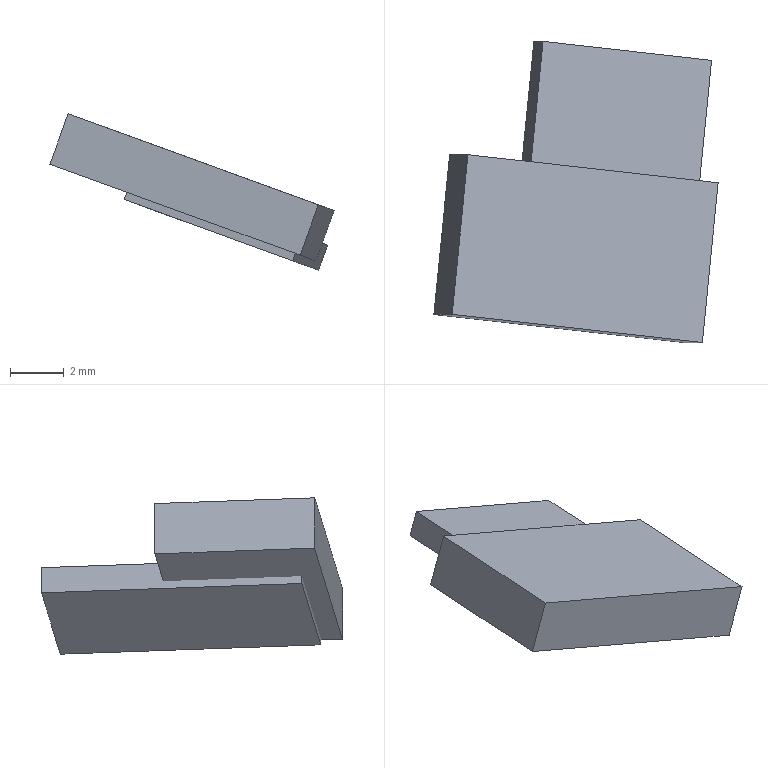Part | 2 solids | 12 faces | volume 185.884 mm3 | plane 12